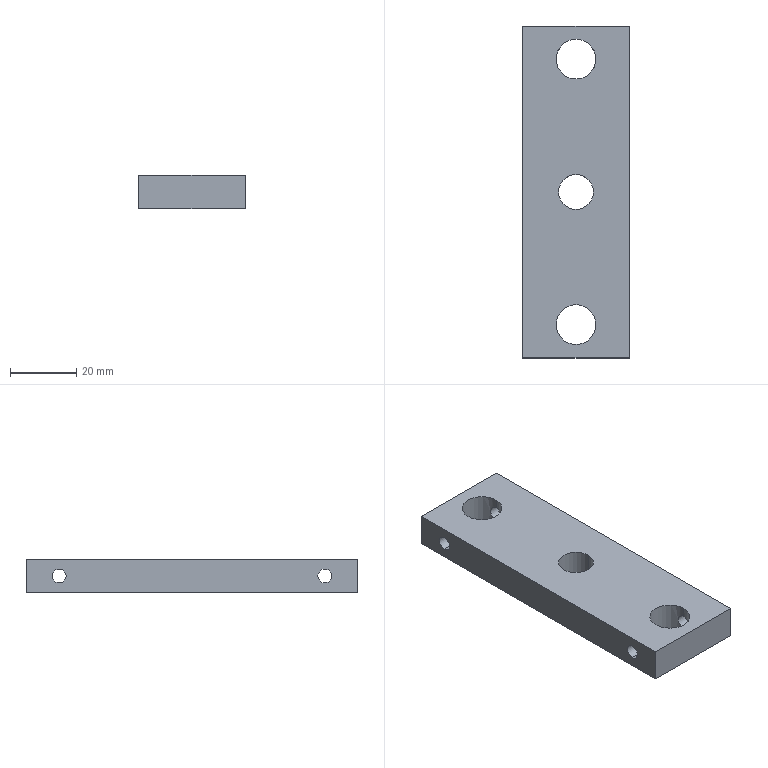Part | STEP file | X77b-01010a | 1 solid | 62 faces | box 32 x 100 x 10 mm | volume 27866 mm3 | cylinder 38 | cone 12 | plane 12 | commonest cylinder face diameters 2.5 x8 3 x8 4.2 x8 3.3 x4 4 x4 12 x4